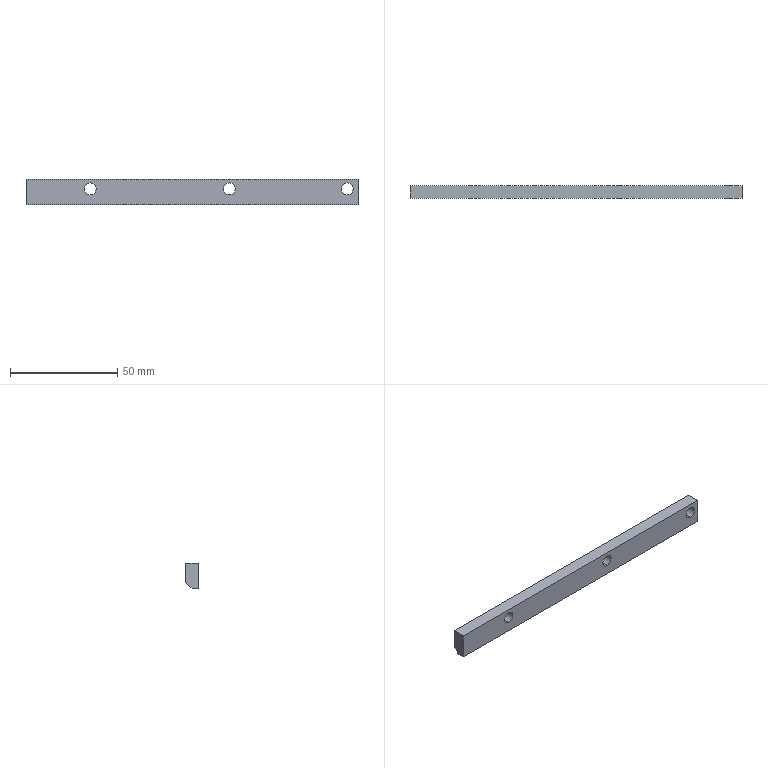Part | STEP file | cover plate 4 | 1 solid | 13 faces | box 155 x 6 x 12 mm | volume 10035 mm3 | plane 7 | cylinder 6 | commonest cylinder face diameters 5.5 x6
STEP:
#1=CARTESIAN_POINT('',(0.,0.,0.));
#2=DIRECTION('',(0.,0.,1.));
#3=DIRECTION('',(1.,0.,0.));
#4=AXIS2_PLACEMENT_3D('',#1,#2,#3);
#5=CARTESIAN_POINT('',(-34.258,0.,9.25));
#6=VERTEX_POINT('',#5);
#7=CARTESIAN_POINT('',(-34.258,6.,9.25));
#8=VERTEX_POINT('',#7);
#9=CARTESIAN_POINT('',(-34.258,6.,9.25));
#10=DIRECTION('',(0.,1.,0.));
#11=VECTOR('',#10,1.);
#12=LINE('',#9,#11);
#13=CARTESIAN_POINT('',(-34.258,6.,6.5));
#14=DIRECTION('',(0.,1.,0.));
#15=DIRECTION('',(0.,0.,1.));
#16=AXIS2_PLACEMENT_3D('',#13,#14,#15);
#17=CYLINDRICAL_SURFACE('',#16,2.75);
#18=CARTESIAN_POINT('',(6.283,0.));
#19=DIRECTION('',(0.,1.));
#20=VECTOR('',#19,1.);
#21=LINE('',#18,#20);
#22=(GEOMETRIC_REPRESENTATION_CONTEXT(2)PARAMETRIC_REPRESENTATION_CONTEXT()REPRESENTATION_CONTEXT('',''));
#23=DEFINITIONAL_REPRESENTATION('',(#21),#22);
#24=PCURVE('',#17,#23);
#25=CARTESIAN_POINT('',(-34.258,6.,6.5));
#26=DIRECTION('',(0.,1.,0.));
#27=DIRECTION('',(0.,0.,1.));
#28=AXIS2_PLACEMENT_3D('',#25,#26,#27);
#29=CYLINDRICAL_SURFACE('',#28,2.75);
#30=CARTESIAN_POINT('',(0.,0.));
#31=DIRECTION('',(0.,1.));
#32=VECTOR('',#31,1.);
#33=LINE('',#30,#32);
#34=(GEOMETRIC_REPRESENTATION_CONTEXT(2)PARAMETRIC_REPRESENTATION_CONTEXT()REPRESENTATION_CONTEXT('',''));
#35=DEFINITIONAL_REPRESENTATION('',(#33),#34);
#36=PCURVE('',#29,#35);
#37=SURFACE_CURVE('',#12,(#24,#36),.PCURVE_S1.);
#38=EDGE_CURVE('',#6,#8,#37,.T.);
#39=ORIENTED_EDGE('',*,*,#38,.T.);
#40=CARTESIAN_POINT('',(-34.258,6.,3.75));
#41=VERTEX_POINT('',#40);
#42=CARTESIAN_POINT('',(-34.258,6.,6.5));
#43=DIRECTION('',(0.,1.,0.));
#44=DIRECTION('',(0.,0.,1.));
#45=AXIS2_PLACEMENT_3D('',#42,#43,#44);
#46=CIRCLE('',#45,2.75);
#47=CARTESIAN_POINT('',(0.,0.));
#48=DIRECTION('',(1.,0.));
#49=VECTOR('',#48,1.);
#50=LINE('',#47,#49);
#51=(GEOMETRIC_REPRESENTATION_CONTEXT(2)PARAMETRIC_REPRESENTATION_CONTEXT()REPRESENTATION_CONTEXT('',''));
#52=DEFINITIONAL_REPRESENTATION('',(#50),#51);
#53=PCURVE('',#17,#52);
#54=CARTESIAN_POINT('',(15.742,6.,11.));
#55=DIRECTION('',(0.,1.,0.));
#56=DIRECTION('',(0.,0.,1.));
#57=AXIS2_PLACEMENT_3D('',#54,#55,#56);
#58=PLANE('',#57);
#59=CARTESIAN_POINT('',(-4.5,-50.));
#60=DIRECTION('',(1.,0.));
#61=AXIS2_PLACEMENT_2D('',#59,#60);
#62=CIRCLE('',#61,2.75);
#63=(GEOMETRIC_REPRESENTATION_CONTEXT(2)PARAMETRIC_REPRESENTATION_CONTEXT()REPRESENTATION_CONTEXT('',''));
#64=DEFINITIONAL_REPRESENTATION('',(#62),#63);
#65=PCURVE('',#58,#64);
#66=SURFACE_CURVE('',#46,(#53,#65),.PCURVE_S1.);
#67=EDGE_CURVE('',#41,#8,#66,.T.);
#68=ORIENTED_EDGE('',*,*,#67,.F.);
#69=CARTESIAN_POINT('',(-34.258,0.,3.75));
#70=VERTEX_POINT('',#69);
#71=CARTESIAN_POINT('',(-34.258,6.,3.75));
#72=DIRECTION('',(0.,1.,0.));
#73=VECTOR('',#72,1.);
#74=LINE('',#71,#73);
#75=CARTESIAN_POINT('',(3.142,0.));
#76=DIRECTION('',(0.,1.));
#77=VECTOR('',#76,1.);
#78=LINE('',#75,#77);
#79=(GEOMETRIC_REPRESENTATION_CONTEXT(2)PARAMETRIC_REPRESENTATION_CONTEXT()REPRESENTATION_CONTEXT('',''));
#80=DEFINITIONAL_REPRESENTATION('',(#78),#79);
#81=PCURVE('',#17,#80);
#82=CARTESIAN_POINT('',(3.142,0.));
#83=DIRECTION('',(0.,1.));
#84=VECTOR('',#83,1.);
#85=LINE('',#82,#84);
#86=(GEOMETRIC_REPRESENTATION_CONTEXT(2)PARAMETRIC_REPRESENTATION_CONTEXT()REPRESENTATION_CONTEXT('',''));
#87=DEFINITIONAL_REPRESENTATION('',(#85),#86);
#88=PCURVE('',#29,#87);
#89=SURFACE_CURVE('',#74,(#81,#88),.PCURVE_S1.);
#90=EDGE_CURVE('',#70,#41,#89,.T.);
#91=ORIENTED_EDGE('',*,*,#90,.F.);
#92=CARTESIAN_POINT('',(-34.258,0.,6.5));
#93=DIRECTION('',(0.,1.,0.));
#94=DIRECTION('',(0.,0.,1.));
#95=AXIS2_PLACEMENT_3D('',#92,#93,#94);
#96=CIRCLE('',#95,2.75);
#97=CARTESIAN_POINT('',(0.,-6.));
#98=DIRECTION('',(1.,0.));
#99=VECTOR('',#98,1.);
#100=LINE('',#97,#99);
#101=(GEOMETRIC_REPRESENTATION_CONTEXT(2)PARAMETRIC_REPRESENTATION_CONTEXT()REPRESENTATION_CONTEXT('',''));
#102=DEFINITIONAL_REPRESENTATION('',(#100),#101);
#103=PCURVE('',#17,#102);
#104=CARTESIAN_POINT('',(15.742,0.,11.));
#105=DIRECTION('',(0.,1.,0.));
#106=DIRECTION('',(0.,0.,1.));
#107=AXIS2_PLACEMENT_3D('',#104,#105,#106);
#108=PLANE('',#107);
#109=CARTESIAN_POINT('',(-4.5,-50.));
#110=DIRECTION('',(1.,0.));
#111=AXIS2_PLACEMENT_2D('',#109,#110);
#112=CIRCLE('',#111,2.75);
#113=(GEOMETRIC_REPRESENTATION_CONTEXT(2)PARAMETRIC_REPRESENTATION_CONTEXT()REPRESENTATION_CONTEXT('',''));
#114=DEFINITIONAL_REPRESENTATION('',(#112),#113);
#115=PCURVE('',#108,#114);
#116=SURFACE_CURVE('',#96,(#103,#115),.PCURVE_S1.);
#117=EDGE_CURVE('',#70,#6,#116,.T.);
#118=ORIENTED_EDGE('',*,*,#117,.T.);
#119=EDGE_LOOP('',(#39,#68,#91,#118));
#120=FACE_BOUND('',#119,.F.);
#121=ADVANCED_FACE('',(#120),#17,.F.);
#122=CARTESIAN_POINT('',(85.742,0.,9.25));
#123=VERTEX_POINT('',#122);
#124=CARTESIAN_POINT('',(85.742,6.,9.25));
#125=VERTEX_POINT('',#124);
#126=CARTESIAN_POINT('',(85.742,6.,9.25));
#127=DIRECTION('',(0.,1.,0.));
#128=VECTOR('',#127,1.);
#129=LINE('',#126,#128);
#130=CARTESIAN_POINT('',(85.742,6.,6.5));
#131=DIRECTION('',(0.,1.,0.));
#132=DIRECTION('',(0.,0.,1.));
#133=AXIS2_PLACEMENT_3D('',#130,#131,#132);
#134=CYLINDRICAL_SURFACE('',#133,2.75);
#135=CARTESIAN_POINT('',(6.283,0.));
#136=DIRECTION('',(0.,1.));
#137=VECTOR('',#136,1.);
#138=LINE('',#135,#137);
#139=(GEOMETRIC_REPRESENTATION_CONTEXT(2)PARAMETRIC_REPRESENTATION_CONTEXT()REPRESENTATION_CONTEXT('',''));
#140=DEFINITIONAL_REPRESENTATION('',(#138),#139);
#141=PCURVE('',#134,#140);
#142=CARTESIAN_POINT('',(85.742,6.,6.5));
#143=DIRECTION('',(0.,1.,0.));
#144=DIRECTION('',(0.,0.,1.));
#145=AXIS2_PLACEMENT_3D('',#142,#143,#144);
#146=CYLINDRICAL_SURFACE('',#145,2.75);
#147=CARTESIAN_POINT('',(0.,0.));
#148=DIRECTION('',(0.,1.));
#149=VECTOR('',#148,1.);
#150=LINE('',#147,#149);
#151=(GEOMETRIC_REPRESENTATION_CONTEXT(2)PARAMETRIC_REPRESENTATION_CONTEXT()REPRESENTATION_CONTEXT('',''));
#152=DEFINITIONAL_REPRESENTATION('',(#150),#151);
#153=PCURVE('',#146,#152);
#154=SURFACE_CURVE('',#129,(#141,#153),.PCURVE_S1.);
#155=EDGE_CURVE('',#123,#125,#154,.T.);
#156=ORIENTED_EDGE('',*,*,#155,.T.);
#157=CARTESIAN_POINT('',(85.742,6.,3.75));
#158=VERTEX_POINT('',#157);
#159=CARTESIAN_POINT('',(85.742,6.,6.5));
#160=DIRECTION('',(0.,1.,0.));
#161=DIRECTION('',(0.,0.,1.));
#162=AXIS2_PLACEMENT_3D('',#159,#160,#161);
#163=CIRCLE('',#162,2.75);
#164=CARTESIAN_POINT('',(0.,0.));
#165=DIRECTION('',(1.,0.));
#166=VECTOR('',#165,1.);
#167=LINE('',#164,#166);
#168=(GEOMETRIC_REPRESENTATION_CONTEXT(2)PARAMETRIC_REPRESENTATION_CONTEXT()REPRESENTATION_CONTEXT('',''));
#169=DEFINITIONAL_REPRESENTATION('',(#167),#168);
#170=PCURVE('',#134,#169);
#171=CARTESIAN_POINT('',(-4.5,70.));
#172=DIRECTION('',(1.,0.));
#173=AXIS2_PLACEMENT_2D('',#171,#172);
#174=CIRCLE('',#173,2.75);
#175=(GEOMETRIC_REPRESENTATION_CONTEXT(2)PARAMETRIC_REPRESENTATION_CONTEXT()REPRESENTATION_CONTEXT('',''));
#176=DEFINITIONAL_REPRESENTATION('',(#174),#175);
#177=PCURVE('',#58,#176);
#178=SURFACE_CURVE('',#163,(#170,#177),.PCURVE_S1.);
#179=EDGE_CURVE('',#158,#125,#178,.T.);
#180=ORIENTED_EDGE('',*,*,#179,.F.);
#181=CARTESIAN_POINT('',(85.742,0.,3.75));
#182=VERTEX_POINT('',#181);
#183=CARTESIAN_POINT('',(85.742,6.,3.75));
#184=DIRECTION('',(0.,1.,0.));
#185=VECTOR('',#184,1.);
#186=LINE('',#183,#185);
#187=CARTESIAN_POINT('',(3.142,0.));
#188=DIRECTION('',(0.,1.));
#189=VECTOR('',#188,1.);
#190=LINE('',#187,#189);
#191=(GEOMETRIC_REPRESENTATION_CONTEXT(2)PARAMETRIC_REPRESENTATION_CONTEXT()REPRESENTATION_CONTEXT('',''));
#192=DEFINITIONAL_REPRESENTATION('',(#190),#191);
#193=PCURVE('',#134,#192);
#194=CARTESIAN_POINT('',(3.142,0.));
#195=DIRECTION('',(0.,1.));
#196=VECTOR('',#195,1.);
#197=LINE('',#194,#196);
#198=(GEOMETRIC_REPRESENTATION_CONTEXT(2)PARAMETRIC_REPRESENTATION_CONTEXT()REPRESENTATION_CONTEXT('',''));
#199=DEFINITIONAL_REPRESENTATION('',(#197),#198);
#200=PCURVE('',#146,#199);
#201=SURFACE_CURVE('',#186,(#193,#200),.PCURVE_S1.);
#202=EDGE_CURVE('',#182,#158,#201,.T.);
#203=ORIENTED_EDGE('',*,*,#202,.F.);
#204=CARTESIAN_POINT('',(85.742,0.,6.5));
#205=DIRECTION('',(0.,1.,0.));
#206=DIRECTION('',(0.,0.,1.));
#207=AXIS2_PLACEMENT_3D('',#204,#205,#206);
#208=CIRCLE('',#207,2.75);
#209=CARTESIAN_POINT('',(0.,-6.));
#210=DIRECTION('',(1.,0.));
#211=VECTOR('',#210,1.);
#212=LINE('',#209,#211);
#213=(GEOMETRIC_REPRESENTATION_CONTEXT(2)PARAMETRIC_REPRESENTATION_CONTEXT()REPRESENTATION_CONTEXT('',''));
#214=DEFINITIONAL_REPRESENTATION('',(#212),#213);
#215=PCURVE('',#134,#214);
#216=CARTESIAN_POINT('',(-4.5,70.));
#217=DIRECTION('',(1.,0.));
#218=AXIS2_PLACEMENT_2D('',#216,#217);
#219=CIRCLE('',#218,2.75);
#220=(GEOMETRIC_REPRESENTATION_CONTEXT(2)PARAMETRIC_REPRESENTATION_CONTEXT()REPRESENTATION_CONTEXT('',''));
#221=DEFINITIONAL_REPRESENTATION('',(#219),#220);
#222=PCURVE('',#108,#221);
#223=SURFACE_CURVE('',#208,(#215,#222),.PCURVE_S1.);
#224=EDGE_CURVE('',#182,#123,#223,.T.);
#225=ORIENTED_EDGE('',*,*,#224,.T.);
#226=EDGE_LOOP('',(#156,#180,#203,#225));
#227=FACE_BOUND('',#226,.F.);
#228=ADVANCED_FACE('',(#227),#134,.F.);
#229=CARTESIAN_POINT('',(30.742,0.,9.25));
#230=VERTEX_POINT('',#229);
#231=CARTESIAN_POINT('',(30.742,6.,9.25));
#232=VERTEX_POINT('',#231);
#233=CARTESIAN_POINT('',(30.742,6.,9.25));
#234=DIRECTION('',(0.,1.,0.));
#235=VECTOR('',#234,1.);
#236=LINE('',#233,#235);
#237=CARTESIAN_POINT('',(30.742,6.,6.5));
#238=DIRECTION('',(0.,1.,0.));
#239=DIRECTION('',(0.,0.,1.));
#240=AXIS2_PLACEMENT_3D('',#237,#238,#239);
#241=CYLINDRICAL_SURFACE('',#240,2.75);
#242=CARTESIAN_POINT('',(6.283,0.));
#243=DIRECTION('',(0.,1.));
#244=VECTOR('',#243,1.);
#245=LINE('',#242,#244);
#246=(GEOMETRIC_REPRESENTATION_CONTEXT(2)PARAMETRIC_REPRESENTATION_CONTEXT()REPRESENTATION_CONTEXT('',''));
#247=DEFINITIONAL_REPRESENTATION('',(#245),#246);
#248=PCURVE('',#241,#247);
#249=CARTESIAN_POINT('',(30.742,6.,6.5));
#250=DIRECTION('',(0.,1.,0.));
#251=DIRECTION('',(0.,0.,1.));
#252=AXIS2_PLACEMENT_3D('',#249,#250,#251);
#253=CYLINDRICAL_SURFACE('',#252,2.75);
#254=CARTESIAN_POINT('',(0.,0.));
#255=DIRECTION('',(0.,1.));
#256=VECTOR('',#255,1.);
#257=LINE('',#254,#256);
#258=(GEOMETRIC_REPRESENTATION_CONTEXT(2)PARAMETRIC_REPRESENTATION_CONTEXT()REPRESENTATION_CONTEXT('',''));
#259=DEFINITIONAL_REPRESENTATION('',(#257),#258);
#260=PCURVE('',#253,#259);
#261=SURFACE_CURVE('',#236,(#248,#260),.PCURVE_S1.);
#262=EDGE_CURVE('',#230,#232,#261,.T.);
#263=ORIENTED_EDGE('',*,*,#262,.T.);
#264=CARTESIAN_POINT('',(30.742,6.,3.75));
#265=VERTEX_POINT('',#264);
#266=CARTESIAN_POINT('',(30.742,6.,6.5));
#267=DIRECTION('',(0.,1.,0.));
#268=DIRECTION('',(0.,0.,1.));
#269=AXIS2_PLACEMENT_3D('',#266,#267,#268);
#270=CIRCLE('',#269,2.75);
#271=CARTESIAN_POINT('',(0.,0.));
#272=DIRECTION('',(1.,0.));
#273=VECTOR('',#272,1.);
#274=LINE('',#271,#273);
#275=(GEOMETRIC_REPRESENTATION_CONTEXT(2)PARAMETRIC_REPRESENTATION_CONTEXT()REPRESENTATION_CONTEXT('',''));
#276=DEFINITIONAL_REPRESENTATION('',(#274),#275);
#277=PCURVE('',#241,#276);
#278=CARTESIAN_POINT('',(-4.5,15.));
#279=DIRECTION('',(1.,0.));
#280=AXIS2_PLACEMENT_2D('',#278,#279);
#281=CIRCLE('',#280,2.75);
#282=(GEOMETRIC_REPRESENTATION_CONTEXT(2)PARAMETRIC_REPRESENTATION_CONTEXT()REPRESENTATION_CONTEXT('',''));
#283=DEFINITIONAL_REPRESENTATION('',(#281),#282);
#284=PCURVE('',#58,#283);
#285=SURFACE_CURVE('',#270,(#277,#284),.PCURVE_S1.);
#286=EDGE_CURVE('',#265,#232,#285,.T.);
#287=ORIENTED_EDGE('',*,*,#286,.F.);
#288=CARTESIAN_POINT('',(30.742,0.,3.75));
#289=VERTEX_POINT('',#288);
#290=CARTESIAN_POINT('',(30.742,6.,3.75));
#291=DIRECTION('',(0.,1.,0.));
#292=VECTOR('',#291,1.);
#293=LINE('',#290,#292);
#294=CARTESIAN_POINT('',(3.142,0.));
#295=DIRECTION('',(0.,1.));
#296=VECTOR('',#295,1.);
#297=LINE('',#294,#296);
#298=(GEOMETRIC_REPRESENTATION_CONTEXT(2)PARAMETRIC_REPRESENTATION_CONTEXT()REPRESENTATION_CONTEXT('',''));
#299=DEFINITIONAL_REPRESENTATION('',(#297),#298);
#300=PCURVE('',#241,#299);
#301=CARTESIAN_POINT('',(3.142,0.));
#302=DIRECTION('',(0.,1.));
#303=VECTOR('',#302,1.);
#304=LINE('',#301,#303);
#305=(GEOMETRIC_REPRESENTATION_CONTEXT(2)PARAMETRIC_REPRESENTATION_CONTEXT()REPRESENTATION_CONTEXT('',''));
#306=DEFINITIONAL_REPRESENTATION('',(#304),#305);
#307=PCURVE('',#253,#306);
#308=SURFACE_CURVE('',#293,(#300,#307),.PCURVE_S1.);
#309=EDGE_CURVE('',#289,#265,#308,.T.);
#310=ORIENTED_EDGE('',*,*,#309,.F.);
#311=CARTESIAN_POINT('',(30.742,0.,6.5));
#312=DIRECTION('',(0.,1.,0.));
#313=DIRECTION('',(0.,0.,1.));
#314=AXIS2_PLACEMENT_3D('',#311,#312,#313);
#315=CIRCLE('',#314,2.75);
#316=CARTESIAN_POINT('',(0.,-6.));
#317=DIRECTION('',(1.,0.));
#318=VECTOR('',#317,1.);
#319=LINE('',#316,#318);
#320=(GEOMETRIC_REPRESENTATION_CONTEXT(2)PARAMETRIC_REPRESENTATION_CONTEXT()REPRESENTATION_CONTEXT('',''));
#321=DEFINITIONAL_REPRESENTATION('',(#319),#320);
#322=PCURVE('',#241,#321);
#323=CARTESIAN_POINT('',(-4.5,15.));
#324=DIRECTION('',(1.,0.));
#325=AXIS2_PLACEMENT_2D('',#323,#324);
#326=CIRCLE('',#325,2.75);
#327=(GEOMETRIC_REPRESENTATION_CONTEXT(2)PARAMETRIC_REPRESENTATION_CONTEXT()REPRESENTATION_CONTEXT('',''));
#328=DEFINITIONAL_REPRESENTATION('',(#326),#327);
#329=PCURVE('',#108,#328);
#330=SURFACE_CURVE('',#315,(#322,#329),.PCURVE_S1.);
#331=EDGE_CURVE('',#289,#230,#330,.T.);
#332=ORIENTED_EDGE('',*,*,#331,.T.);
#333=EDGE_LOOP('',(#263,#287,#310,#332));
#334=FACE_BOUND('',#333,.F.);
#335=ADVANCED_FACE('',(#334),#241,.F.);
#336=CARTESIAN_POINT('',(-64.258,0.,11.));
#337=VERTEX_POINT('',#336);
#338=CARTESIAN_POINT('',(90.742,0.,11.));
#339=VERTEX_POINT('',#338);
#340=CARTESIAN_POINT('',(15.742,0.,11.));
#341=DIRECTION('',(1.,0.,0.));
#342=VECTOR('',#341,1.);
#343=LINE('',#340,#342);
#344=CARTESIAN_POINT('',(15.742,6.,11.));
#345=DIRECTION('',(0.,0.,-1.));
#346=DIRECTION('',(-1.,0.,0.));
#347=AXIS2_PLACEMENT_3D('',#344,#345,#346);
#348=PLANE('',#347);
#349=CARTESIAN_POINT('',(0.,-6.));
#350=DIRECTION('',(-1.,0.));
#351=VECTOR('',#350,1.);
#352=LINE('',#349,#351);
#353=(GEOMETRIC_REPRESENTATION_CONTEXT(2)PARAMETRIC_REPRESENTATION_CONTEXT()REPRESENTATION_CONTEXT('',''));
#354=DEFINITIONAL_REPRESENTATION('',(#352),#353);
#355=PCURVE('',#348,#354);
#356=CARTESIAN_POINT('',(0.,0.));
#357=DIRECTION('',(0.,1.));
#358=VECTOR('',#357,1.);
#359=LINE('',#356,#358);
#360=(GEOMETRIC_REPRESENTATION_CONTEXT(2)PARAMETRIC_REPRESENTATION_CONTEXT()REPRESENTATION_CONTEXT('',''));
#361=DEFINITIONAL_REPRESENTATION('',(#359),#360);
#362=PCURVE('',#108,#361);
#363=SURFACE_CURVE('',#343,(#355,#362),.PCURVE_S1.);
#364=EDGE_CURVE('',#337,#339,#363,.T.);
#365=ORIENTED_EDGE('',*,*,#364,.T.);
#366=CARTESIAN_POINT('',(90.742,6.,11.));
#367=VERTEX_POINT('',#366);
#368=CARTESIAN_POINT('',(90.742,6.,11.));
#369=DIRECTION('',(0.,-1.,0.));
#370=VECTOR('',#369,1.);
#371=LINE('',#368,#370);
#372=CARTESIAN_POINT('',(-75.,0.));
#373=DIRECTION('',(0.,-1.));
#374=VECTOR('',#373,1.);
#375=LINE('',#372,#374);
#376=(GEOMETRIC_REPRESENTATION_CONTEXT(2)PARAMETRIC_REPRESENTATION_CONTEXT()REPRESENTATION_CONTEXT('',''));
#377=DEFINITIONAL_REPRESENTATION('',(#375),#376);
#378=PCURVE('',#348,#377);
#379=CARTESIAN_POINT('',(90.742,0.,-1.));
#380=DIRECTION('',(1.,0.,0.));
#381=DIRECTION('',(0.,0.,-1.));
#382=AXIS2_PLACEMENT_3D('',#379,#380,#381);
#383=PLANE('',#382);
#384=CARTESIAN_POINT('',(-12.,6.));
#385=DIRECTION('',(0.,-1.));
#386=VECTOR('',#385,1.);
#387=LINE('',#384,#386);
#388=(GEOMETRIC_REPRESENTATION_CONTEXT(2)PARAMETRIC_REPRESENTATION_CONTEXT()REPRESENTATION_CONTEXT('',''));
#389=DEFINITIONAL_REPRESENTATION('',(#387),#388);
#390=PCURVE('',#383,#389);
#391=SURFACE_CURVE('',#371,(#378,#390),.PCURVE_S1.);
#392=EDGE_CURVE('',#367,#339,#391,.T.);
#393=ORIENTED_EDGE('',*,*,#392,.F.);
#394=CARTESIAN_POINT('',(-64.258,6.,11.));
#395=VERTEX_POINT('',#394);
#396=CARTESIAN_POINT('',(15.742,6.,11.));
#397=DIRECTION('',(1.,0.,0.));
#398=VECTOR('',#397,1.);
#399=LINE('',#396,#398);
#400=CARTESIAN_POINT('',(0.,0.));
#401=DIRECTION('',(-1.,0.));
#402=VECTOR('',#401,1.);
#403=LINE('',#400,#402);
#404=(GEOMETRIC_REPRESENTATION_CONTEXT(2)PARAMETRIC_REPRESENTATION_CONTEXT()REPRESENTATION_CONTEXT('',''));
#405=DEFINITIONAL_REPRESENTATION('',(#403),#404);
#406=PCURVE('',#348,#405);
#407=CARTESIAN_POINT('',(0.,0.));
#408=DIRECTION('',(0.,1.));
#409=VECTOR('',#408,1.);
#410=LINE('',#407,#409);
#411=(GEOMETRIC_REPRESENTATION_CONTEXT(2)PARAMETRIC_REPRESENTATION_CONTEXT()REPRESENTATION_CONTEXT('',''));
#412=DEFINITIONAL_REPRESENTATION('',(#410),#411);
#413=PCURVE('',#58,#412);
#414=SURFACE_CURVE('',#399,(#406,#413),.PCURVE_S1.);
#415=EDGE_CURVE('',#395,#367,#414,.T.);
#416=ORIENTED_EDGE('',*,*,#415,.F.);
#417=CARTESIAN_POINT('',(-64.258,0.,11.));
#418=DIRECTION('',(0.,1.,0.));
#419=VECTOR('',#418,1.);
#420=LINE('',#417,#419);
#421=CARTESIAN_POINT('',(80.,-6.));
#422=DIRECTION('',(0.,1.));
#423=VECTOR('',#422,1.);
#424=LINE('',#421,#423);
#425=(GEOMETRIC_REPRESENTATION_CONTEXT(2)PARAMETRIC_REPRESENTATION_CONTEXT()REPRESENTATION_CONTEXT('',''));
#426=DEFINITIONAL_REPRESENTATION('',(#424),#425);
#427=PCURVE('',#348,#426);
#428=CARTESIAN_POINT('',(-64.258,6.,11.));
#429=DIRECTION('',(-1.,0.,0.));
#430=DIRECTION('',(0.,0.,1.));
#431=AXIS2_PLACEMENT_3D('',#428,#429,#430);
#432=PLANE('',#431);
#433=CARTESIAN_POINT('',(0.,-6.));
#434=DIRECTION('',(0.,1.));
#435=VECTOR('',#434,1.);
#436=LINE('',#433,#435);
#437=(GEOMETRIC_REPRESENTATION_CONTEXT(2)PARAMETRIC_REPRESENTATION_CONTEXT()REPRESENTATION_CONTEXT('',''));
#438=DEFINITIONAL_REPRESENTATION('',(#436),#437);
#439=PCURVE('',#432,#438);
#440=SURFACE_CURVE('',#420,(#427,#439),.PCURVE_S1.);
#441=EDGE_CURVE('',#337,#395,#440,.T.);
#442=ORIENTED_EDGE('',*,*,#441,.F.);
#443=EDGE_LOOP('',(#365,#393,#416,#442));
#444=FACE_BOUND('',#443,.T.);
#445=ADVANCED_FACE('',(#444),#348,.F.);
#446=CARTESIAN_POINT('',(90.742,0.,-1.));
#447=VERTEX_POINT('',#446);
#448=CARTESIAN_POINT('',(-64.258,0.,-1.));
#449=VERTEX_POINT('',#448);
#450=CARTESIAN_POINT('',(15.742,0.,-1.));
#451=DIRECTION('',(-1.,0.,0.));
#452=VECTOR('',#451,1.);
#453=LINE('',#450,#452);
#454=CARTESIAN_POINT('',(15.742,6.,-1.));
#455=DIRECTION('',(0.,0.,1.));
#456=DIRECTION('',(1.,0.,0.));
#457=AXIS2_PLACEMENT_3D('',#454,#455,#456);
#458=PLANE('',#457);
#459=CARTESIAN_POINT('',(0.,-6.));
#460=DIRECTION('',(-1.,0.));
#461=VECTOR('',#460,1.);
#462=LINE('',#459,#461);
#463=(GEOMETRIC_REPRESENTATION_CONTEXT(2)PARAMETRIC_REPRESENTATION_CONTEXT()REPRESENTATION_CONTEXT('',''));
#464=DEFINITIONAL_REPRESENTATION('',(#462),#463);
#465=PCURVE('',#458,#464);
#466=CARTESIAN_POINT('',(-12.,0.));
#467=DIRECTION('',(0.,-1.));
#468=VECTOR('',#467,1.);
#469=LINE('',#466,#468);
#470=(GEOMETRIC_REPRESENTATION_CONTEXT(2)PARAMETRIC_REPRESENTATION_CONTEXT()REPRESENTATION_CONTEXT('',''));
#471=DEFINITIONAL_REPRESENTATION('',(#469),#470);
#472=PCURVE('',#108,#471);
#473=SURFACE_CURVE('',#453,(#465,#472),.PCURVE_S1.);
#474=EDGE_CURVE('',#447,#449,#473,.T.);
#475=ORIENTED_EDGE('',*,*,#474,.T.);
#476=CARTESIAN_POINT('',(-64.258,3.,-1.));
#477=VERTEX_POINT('',#476);
#478=CARTESIAN_POINT('',(-64.258,3.,-1.));
#479=DIRECTION('',(0.,-1.,0.));
#480=VECTOR('',#479,1.);
#481=LINE('',#478,#480);
#482=CARTESIAN_POINT('',(-80.,-3.));
#483=DIRECTION('',(0.,-1.));
#484=VECTOR('',#483,1.);
#485=LINE('',#482,#484);
#486=(GEOMETRIC_REPRESENTATION_CONTEXT(2)PARAMETRIC_REPRESENTATION_CONTEXT()REPRESENTATION_CONTEXT('',''));
#487=DEFINITIONAL_REPRESENTATION('',(#485),#486);
#488=PCURVE('',#458,#487);
#489=CARTESIAN_POINT('',(-12.,-3.));
#490=DIRECTION('',(0.,-1.));
#491=VECTOR('',#490,1.);
#492=LINE('',#489,#491);
#493=(GEOMETRIC_REPRESENTATION_CONTEXT(2)PARAMETRIC_REPRESENTATION_CONTEXT()REPRESENTATION_CONTEXT('',''));
#494=DEFINITIONAL_REPRESENTATION('',(#492),#493);
#495=PCURVE('',#432,#494);
#496=SURFACE_CURVE('',#481,(#488,#495),.PCURVE_S1.);
#497=EDGE_CURVE('',#477,#449,#496,.T.);
#498=ORIENTED_EDGE('',*,*,#497,.F.);
#499=CARTESIAN_POINT('',(90.742,3.,-1.));
#500=VERTEX_POINT('',#499);
#501=CARTESIAN_POINT('',(60.742,3.,-1.));
#502=DIRECTION('',(1.,0.,0.));
#503=VECTOR('',#502,1.);
#504=LINE('',#501,#503);
#505=CARTESIAN_POINT('',(45.,-3.));
#506=DIRECTION('',(1.,0.));
#507=VECTOR('',#506,1.);
#508=LINE('',#505,#507);
#509=(GEOMETRIC_REPRESENTATION_CONTEXT(2)PARAMETRIC_REPRESENTATION_CONTEXT()REPRESENTATION_CONTEXT('',''));
#510=DEFINITIONAL_REPRESENTATION('',(#508),#509);
#511=PCURVE('',#458,#510);
#512=CARTESIAN_POINT('',(15.742,6.,2.));
#513=DIRECTION('',(0.,0.7071,-0.7071));
#514=DIRECTION('',(0.,0.7071,0.7071));
#515=AXIS2_PLACEMENT_3D('',#512,#513,#514);
#516=PLANE('',#515);
#517=CARTESIAN_POINT('',(-4.243,45.));
#518=DIRECTION('',(0.,1.));
#519=VECTOR('',#518,1.);
#520=LINE('',#517,#519);
#521=(GEOMETRIC_REPRESENTATION_CONTEXT(2)PARAMETRIC_REPRESENTATION_CONTEXT()REPRESENTATION_CONTEXT('',''));
#522=DEFINITIONAL_REPRESENTATION('',(#520),#521);
#523=PCURVE('',#516,#522);
#524=SURFACE_CURVE('',#504,(#511,#523),.PCURVE_S1.);
#525=EDGE_CURVE('',#477,#500,#524,.T.);
#526=ORIENTED_EDGE('',*,*,#525,.T.);
#527=CARTESIAN_POINT('',(90.742,0.,-1.));
#528=DIRECTION('',(0.,1.,0.));
#529=VECTOR('',#528,1.);
#530=LINE('',#527,#529);
#531=CARTESIAN_POINT('',(75.,-6.));
#532=DIRECTION('',(0.,1.));
#533=VECTOR('',#532,1.);
#534=LINE('',#531,#533);
#535=(GEOMETRIC_REPRESENTATION_CONTEXT(2)PARAMETRIC_REPRESENTATION_CONTEXT()REPRESENTATION_CONTEXT('',''));
#536=DEFINITIONAL_REPRESENTATION('',(#534),#535);
#537=PCURVE('',#458,#536);
#538=CARTESIAN_POINT('',(0.,0.));
#539=DIRECTION('',(0.,1.));
#540=VECTOR('',#539,1.);
#541=LINE('',#538,#540);
#542=(GEOMETRIC_REPRESENTATION_CONTEXT(2)PARAMETRIC_REPRESENTATION_CONTEXT()REPRESENTATION_CONTEXT('',''));
#543=DEFINITIONAL_REPRESENTATION('',(#541),#542);
#544=PCURVE('',#383,#543);
#545=SURFACE_CURVE('',#530,(#537,#544),.PCURVE_S1.);
#546=EDGE_CURVE('',#447,#500,#545,.T.);
#547=ORIENTED_EDGE('',*,*,#546,.F.);
#548=EDGE_LOOP('',(#475,#498,#526,#547));
#549=FACE_BOUND('',#548,.T.);
#550=ADVANCED_FACE('',(#549),#458,.F.);
#551=CARTESIAN_POINT('',(-34.258,6.,6.5));
#552=DIRECTION('',(0.,1.,0.));
#553=DIRECTION('',(0.,0.,1.));
#554=AXIS2_PLACEMENT_3D('',#551,#552,#553);
#555=CIRCLE('',#554,2.75);
#556=CARTESIAN_POINT('',(-4.5,-50.));
#557=DIRECTION('',(1.,0.));
#558=AXIS2_PLACEMENT_2D('',#556,#557);
#559=CIRCLE('',#558,2.75);
#560=(GEOMETRIC_REPRESENTATION_CONTEXT(2)PARAMETRIC_REPRESENTATION_CONTEXT()REPRESENTATION_CONTEXT('',''));
#561=DEFINITIONAL_REPRESENTATION('',(#559),#560);
#562=PCURVE('',#58,#561);
#563=CARTESIAN_POINT('',(0.,0.));
#564=DIRECTION('',(1.,0.));
#565=VECTOR('',#564,1.);
#566=LINE('',#563,#565);
#567=(GEOMETRIC_REPRESENTATION_CONTEXT(2)PARAMETRIC_REPRESENTATION_CONTEXT()REPRESENTATION_CONTEXT('',''));
#568=DEFINITIONAL_REPRESENTATION('',(#566),#567);
#569=PCURVE('',#29,#568);
#570=SURFACE_CURVE('',#555,(#562,#569),.PCURVE_S1.);
#571=EDGE_CURVE('',#8,#41,#570,.T.);
#572=ORIENTED_EDGE('',*,*,#571,.F.);
#573=ORIENTED_EDGE('',*,*,#67,.F.);
#574=EDGE_LOOP('',(#572,#573));
#575=FACE_BOUND('',#574,.T.);
#576=CARTESIAN_POINT('',(85.742,6.,6.5));
#577=DIRECTION('',(0.,1.,0.));
#578=DIRECTION('',(0.,0.,1.));
#579=AXIS2_PLACEMENT_3D('',#576,#577,#578);
#580=CIRCLE('',#579,2.75);
#581=CARTESIAN_POINT('',(-4.5,70.));
#582=DIRECTION('',(1.,0.));
#583=AXIS2_PLACEMENT_2D('',#581,#582);
#584=CIRCLE('',#583,2.75);
#585=(GEOMETRIC_REPRESENTATION_CONTEXT(2)PARAMETRIC_REPRESENTATION_CONTEXT()REPRESENTATION_CONTEXT('',''));
#586=DEFINITIONAL_REPRESENTATION('',(#584),#585);
#587=PCURVE('',#58,#586);
#588=CARTESIAN_POINT('',(0.,0.));
#589=DIRECTION('',(1.,0.));
#590=VECTOR('',#589,1.);
#591=LINE('',#588,#590);
#592=(GEOMETRIC_REPRESENTATION_CONTEXT(2)PARAMETRIC_REPRESENTATION_CONTEXT()REPRESENTATION_CONTEXT('',''));
#593=DEFINITIONAL_REPRESENTATION('',(#591),#592);
#594=PCURVE('',#146,#593);
#595=SURFACE_CURVE('',#580,(#587,#594),.PCURVE_S1.);
#596=EDGE_CURVE('',#125,#158,#595,.T.);
#597=ORIENTED_EDGE('',*,*,#596,.F.);
#598=ORIENTED_EDGE('',*,*,#179,.F.);
#599=EDGE_LOOP('',(#597,#598));
#600=FACE_BOUND('',#599,.T.);
#601=CARTESIAN_POINT('',(30.742,6.,6.5));
#602=DIRECTION('',(0.,1.,0.));
#603=DIRECTION('',(0.,0.,1.));
#604=AXIS2_PLACEMENT_3D('',#601,#602,#603);
#605=CIRCLE('',#604,2.75);
#606=CARTESIAN_POINT('',(-4.5,15.));
#607=DIRECTION('',(1.,0.));
#608=AXIS2_PLACEMENT_2D('',#606,#607);
#609=CIRCLE('',#608,2.75);
#610=(GEOMETRIC_REPRESENTATION_CONTEXT(2)PARAMETRIC_REPRESENTATION_CONTEXT()REPRESENTATION_CONTEXT('',''));
#611=DEFINITIONAL_REPRESENTATION('',(#609),#610);
#612=PCURVE('',#58,#611);
#613=CARTESIAN_POINT('',(0.,0.));
#614=DIRECTION('',(1.,0.));
#615=VECTOR('',#614,1.);
#616=LINE('',#613,#615);
#617=(GEOMETRIC_REPRESENTATION_CONTEXT(2)PARAMETRIC_REPRESENTATION_CONTEXT()REPRESENTATION_CONTEXT('',''));
#618=DEFINITIONAL_REPRESENTATION('',(#616),#617);
#619=PCURVE('',#253,#618);
#620=SURFACE_CURVE('',#605,(#612,#619),.PCURVE_S1.);
#621=EDGE_CURVE('',#232,#265,#620,.T.);
#622=ORIENTED_EDGE('',*,*,#621,.F.);
#623=ORIENTED_EDGE('',*,*,#286,.F.);
#624=EDGE_LOOP('',(#622,#623));
#625=FACE_BOUND('',#624,.T.);
#626=ORIENTED_EDGE('',*,*,#415,.T.);
#627=CARTESIAN_POINT('',(90.742,6.,2.));
#628=VERTEX_POINT('',#627);
#629=CARTESIAN_POINT('',(90.742,6.,2.));
#630=DIRECTION('',(0.,0.,1.));
#631=VECTOR('',#630,1.);
#632=LINE('',#629,#631);
#633=CARTESIAN_POINT('',(-9.,75.));
#634=DIRECTION('',(1.,0.));
#635=VECTOR('',#634,1.);
#636=LINE('',#633,#635);
#637=(GEOMETRIC_REPRESENTATION_CONTEXT(2)PARAMETRIC_REPRESENTATION_CONTEXT()REPRESENTATION_CONTEXT('',''));
#638=DEFINITIONAL_REPRESENTATION('',(#636),#637);
#639=PCURVE('',#58,#638);
#640=CARTESIAN_POINT('',(-3.,6.));
#641=DIRECTION('',(-1.,0.));
#642=VECTOR('',#641,1.);
#643=LINE('',#640,#642);
#644=(GEOMETRIC_REPRESENTATION_CONTEXT(2)PARAMETRIC_REPRESENTATION_CONTEXT()REPRESENTATION_CONTEXT('',''));
#645=DEFINITIONAL_REPRESENTATION('',(#643),#644);
#646=PCURVE('',#383,#645);
#647=SURFACE_CURVE('',#632,(#639,#646),.PCURVE_S1.);
#648=EDGE_CURVE('',#628,#367,#647,.T.);
#649=ORIENTED_EDGE('',*,*,#648,.F.);
#650=CARTESIAN_POINT('',(-64.258,6.,2.));
#651=VERTEX_POINT('',#650);
#652=CARTESIAN_POINT('',(15.742,6.,2.));
#653=DIRECTION('',(-1.,0.,0.));
#654=VECTOR('',#653,1.);
#655=LINE('',#652,#654);
#656=CARTESIAN_POINT('',(-9.,0.));
#657=DIRECTION('',(0.,-1.));
#658=VECTOR('',#657,1.);
#659=LINE('',#656,#658);
#660=(GEOMETRIC_REPRESENTATION_CONTEXT(2)PARAMETRIC_REPRESENTATION_CONTEXT()REPRESENTATION_CONTEXT('',''));
#661=DEFINITIONAL_REPRESENTATION('',(#659),#660);
#662=PCURVE('',#58,#661);
#663=CARTESIAN_POINT('',(0.,0.));
#664=DIRECTION('',(0.,-1.));
#665=VECTOR('',#664,1.);
#666=LINE('',#663,#665);
#667=(GEOMETRIC_REPRESENTATION_CONTEXT(2)PARAMETRIC_REPRESENTATION_CONTEXT()REPRESENTATION_CONTEXT('',''));
#668=DEFINITIONAL_REPRESENTATION('',(#666),#667);
#669=PCURVE('',#516,#668);
#670=SURFACE_CURVE('',#655,(#662,#669),.PCURVE_S1.);
#671=EDGE_CURVE('',#628,#651,#670,.T.);
#672=ORIENTED_EDGE('',*,*,#671,.T.);
#673=CARTESIAN_POINT('',(-64.258,6.,11.));
#674=DIRECTION('',(0.,0.,-1.));
#675=VECTOR('',#674,1.);
#676=LINE('',#673,#675);
#677=CARTESIAN_POINT('',(0.,-80.));
#678=DIRECTION('',(-1.,0.));
#679=VECTOR('',#678,1.);
#680=LINE('',#677,#679);
#681=(GEOMETRIC_REPRESENTATION_CONTEXT(2)PARAMETRIC_REPRESENTATION_CONTEXT()REPRESENTATION_CONTEXT('',''));
#682=DEFINITIONAL_REPRESENTATION('',(#680),#681);
#683=PCURVE('',#58,#682);
#684=CARTESIAN_POINT('',(0.,0.));
#685=DIRECTION('',(-1.,0.));
#686=VECTOR('',#685,1.);
#687=LINE('',#684,#686);
#688=(GEOMETRIC_REPRESENTATION_CONTEXT(2)PARAMETRIC_REPRESENTATION_CONTEXT()REPRESENTATION_CONTEXT('',''));
#689=DEFINITIONAL_REPRESENTATION('',(#687),#688);
#690=PCURVE('',#432,#689);
#691=SURFACE_CURVE('',#676,(#683,#690),.PCURVE_S1.);
#692=EDGE_CURVE('',#395,#651,#691,.T.);
#693=ORIENTED_EDGE('',*,*,#692,.F.);
#694=EDGE_LOOP('',(#626,#649,#672,#693));
#695=FACE_BOUND('',#694,.T.);
#696=ADVANCED_FACE('',(#575,#600,#625,#695),#58,.T.);
#697=CARTESIAN_POINT('',(-34.258,0.,6.5));
#698=DIRECTION('',(0.,1.,0.));
#699=DIRECTION('',(0.,0.,1.));
#700=AXIS2_PLACEMENT_3D('',#697,#698,#699);
#701=CIRCLE('',#700,2.75);
#702=CARTESIAN_POINT('',(-4.5,-50.));
#703=DIRECTION('',(1.,0.));
#704=AXIS2_PLACEMENT_2D('',#702,#703);
#705=CIRCLE('',#704,2.75);
#706=(GEOMETRIC_REPRESENTATION_CONTEXT(2)PARAMETRIC_REPRESENTATION_CONTEXT()REPRESENTATION_CONTEXT('',''));
#707=DEFINITIONAL_REPRESENTATION('',(#705),#706);
#708=PCURVE('',#108,#707);
#709=CARTESIAN_POINT('',(0.,-6.));
#710=DIRECTION('',(1.,0.));
#711=VECTOR('',#710,1.);
#712=LINE('',#709,#711);
#713=(GEOMETRIC_REPRESENTATION_CONTEXT(2)PARAMETRIC_REPRESENTATION_CONTEXT()REPRESENTATION_CONTEXT('',''));
#714=DEFINITIONAL_REPRESENTATION('',(#712),#713);
#715=PCURVE('',#29,#714);
#716=SURFACE_CURVE('',#701,(#708,#715),.PCURVE_S1.);
#717=EDGE_CURVE('',#6,#70,#716,.T.);
#718=ORIENTED_EDGE('',*,*,#717,.T.);
#719=ORIENTED_EDGE('',*,*,#117,.T.);
#720=EDGE_LOOP('',(#718,#719));
#721=FACE_BOUND('',#720,.T.);
#722=CARTESIAN_POINT('',(85.742,0.,6.5));
#723=DIRECTION('',(0.,1.,0.));
#724=DIRECTION('',(0.,0.,1.));
#725=AXIS2_PLACEMENT_3D('',#722,#723,#724);
#726=CIRCLE('',#725,2.75);
#727=CARTESIAN_POINT('',(-4.5,70.));
#728=DIRECTION('',(1.,0.));
#729=AXIS2_PLACEMENT_2D('',#727,#728);
#730=CIRCLE('',#729,2.75);
#731=(GEOMETRIC_REPRESENTATION_CONTEXT(2)PARAMETRIC_REPRESENTATION_CONTEXT()REPRESENTATION_CONTEXT('',''));
#732=DEFINITIONAL_REPRESENTATION('',(#730),#731);
#733=PCURVE('',#108,#732);
#734=CARTESIAN_POINT('',(0.,-6.));
#735=DIRECTION('',(1.,0.));
#736=VECTOR('',#735,1.);
#737=LINE('',#734,#736);
#738=(GEOMETRIC_REPRESENTATION_CONTEXT(2)PARAMETRIC_REPRESENTATION_CONTEXT()REPRESENTATION_CONTEXT('',''));
#739=DEFINITIONAL_REPRESENTATION('',(#737),#738);
#740=PCURVE('',#146,#739);
#741=SURFACE_CURVE('',#726,(#733,#740),.PCURVE_S1.);
#742=EDGE_CURVE('',#123,#182,#741,.T.);
#743=ORIENTED_EDGE('',*,*,#742,.T.);
#744=ORIENTED_EDGE('',*,*,#224,.T.);
#745=EDGE_LOOP('',(#743,#744));
#746=FACE_BOUND('',#745,.T.);
#747=CARTESIAN_POINT('',(30.742,0.,6.5));
#748=DIRECTION('',(0.,1.,0.));
#749=DIRECTION('',(0.,0.,1.));
#750=AXIS2_PLACEMENT_3D('',#747,#748,#749);
#751=CIRCLE('',#750,2.75);
#752=CARTESIAN_POINT('',(-4.5,15.));
#753=DIRECTION('',(1.,0.));
#754=AXIS2_PLACEMENT_2D('',#752,#753);
#755=CIRCLE('',#754,2.75);
#756=(GEOMETRIC_REPRESENTATION_CONTEXT(2)PARAMETRIC_REPRESENTATION_CONTEXT()REPRESENTATION_CONTEXT('',''));
#757=DEFINITIONAL_REPRESENTATION('',(#755),#756);
#758=PCURVE('',#108,#757);
#759=CARTESIAN_POINT('',(0.,-6.));
#760=DIRECTION('',(1.,0.));
#761=VECTOR('',#760,1.);
#762=LINE('',#759,#761);
#763=(GEOMETRIC_REPRESENTATION_CONTEXT(2)PARAMETRIC_REPRESENTATION_CONTEXT()REPRESENTATION_CONTEXT('',''));
#764=DEFINITIONAL_REPRESENTATION('',(#762),#763);
#765=PCURVE('',#253,#764);
#766=SURFACE_CURVE('',#751,(#758,#765),.PCURVE_S1.);
#767=EDGE_CURVE('',#230,#289,#766,.T.);
#768=ORIENTED_EDGE('',*,*,#767,.T.);
#769=ORIENTED_EDGE('',*,*,#331,.T.);
#770=EDGE_LOOP('',(#768,#769));
#771=FACE_BOUND('',#770,.T.);
#772=ORIENTED_EDGE('',*,*,#364,.F.);
#773=CARTESIAN_POINT('',(-64.258,0.,-1.));
#774=DIRECTION('',(0.,0.,1.));
#775=VECTOR('',#774,1.);
#776=LINE('',#773,#775);
#777=CARTESIAN_POINT('',(-12.,-80.));
#778=DIRECTION('',(1.,0.));
#779=VECTOR('',#778,1.);
#780=LINE('',#777,#779);
#781=(GEOMETRIC_REPRESENTATION_CONTEXT(2)PARAMETRIC_REPRESENTATION_CONTEXT()REPRESENTATION_CONTEXT('',''));
#782=DEFINITIONAL_REPRESENTATION('',(#780),#781);
#783=PCURVE('',#108,#782);
#784=CARTESIAN_POINT('',(-12.,-6.));
#785=DIRECTION('',(1.,0.));
#786=VECTOR('',#785,1.);
#787=LINE('',#784,#786);
#788=(GEOMETRIC_REPRESENTATION_CONTEXT(2)PARAMETRIC_REPRESENTATION_CONTEXT()REPRESENTATION_CONTEXT('',''));
#789=DEFINITIONAL_REPRESENTATION('',(#787),#788);
#790=PCURVE('',#432,#789);
#791=SURFACE_CURVE('',#776,(#783,#790),.PCURVE_S1.);
#792=EDGE_CURVE('',#449,#337,#791,.T.);
#793=ORIENTED_EDGE('',*,*,#792,.F.);
#794=ORIENTED_EDGE('',*,*,#474,.F.);
#795=CARTESIAN_POINT('',(90.742,0.,11.));
#796=DIRECTION('',(0.,0.,-1.));
#797=VECTOR('',#796,1.);
#798=LINE('',#795,#797);
#799=CARTESIAN_POINT('',(0.,75.));
#800=DIRECTION('',(-1.,0.));
#801=VECTOR('',#800,1.);
#802=LINE('',#799,#801);
#803=(GEOMETRIC_REPRESENTATION_CONTEXT(2)PARAMETRIC_REPRESENTATION_CONTEXT()REPRESENTATION_CONTEXT('',''));
#804=DEFINITIONAL_REPRESENTATION('',(#802),#803);
#805=PCURVE('',#108,#804);
#806=CARTESIAN_POINT('',(-12.,0.));
#807=DIRECTION('',(1.,0.));
#808=VECTOR('',#807,1.);
#809=LINE('',#806,#808);
#810=(GEOMETRIC_REPRESENTATION_CONTEXT(2)PARAMETRIC_REPRESENTATION_CONTEXT()REPRESENTATION_CONTEXT('',''));
#811=DEFINITIONAL_REPRESENTATION('',(#809),#810);
#812=PCURVE('',#383,#811);
#813=SURFACE_CURVE('',#798,(#805,#812),.PCURVE_S1.);
#814=EDGE_CURVE('',#339,#447,#813,.T.);
#815=ORIENTED_EDGE('',*,*,#814,.F.);
#816=EDGE_LOOP('',(#772,#793,#794,#815));
#817=FACE_BOUND('',#816,.T.);
#818=ADVANCED_FACE('',(#721,#746,#771,#817),#108,.F.);
#819=ORIENTED_EDGE('',*,*,#671,.F.);
#820=CARTESIAN_POINT('',(90.742,3.,-1.));
#821=DIRECTION('',(0.,0.7071,0.7071));
#822=VECTOR('',#821,1.);
#823=LINE('',#820,#822);
#824=CARTESIAN_POINT('',(-4.243,75.));
#825=DIRECTION('',(1.,0.));
#826=VECTOR('',#825,1.);
#827=LINE('',#824,#826);
#828=(GEOMETRIC_REPRESENTATION_CONTEXT(2)PARAMETRIC_REPRESENTATION_CONTEXT()REPRESENTATION_CONTEXT('',''));
#829=DEFINITIONAL_REPRESENTATION('',(#827),#828);
#830=PCURVE('',#516,#829);
#831=CARTESIAN_POINT('',(0.,3.));
#832=DIRECTION('',(-0.7071,0.7071));
#833=VECTOR('',#832,1.);
#834=LINE('',#831,#833);
#835=(GEOMETRIC_REPRESENTATION_CONTEXT(2)PARAMETRIC_REPRESENTATION_CONTEXT()REPRESENTATION_CONTEXT('',''));
#836=DEFINITIONAL_REPRESENTATION('',(#834),#835);
#837=PCURVE('',#383,#836);
#838=SURFACE_CURVE('',#823,(#830,#837),.PCURVE_S1.);
#839=EDGE_CURVE('',#500,#628,#838,.T.);
#840=ORIENTED_EDGE('',*,*,#839,.F.);
#841=ORIENTED_EDGE('',*,*,#525,.F.);
#842=CARTESIAN_POINT('',(-64.258,6.,2.));
#843=DIRECTION('',(0.,-0.7071,-0.7071));
#844=VECTOR('',#843,1.);
#845=LINE('',#842,#844);
#846=CARTESIAN_POINT('',(0.,-80.));
#847=DIRECTION('',(-1.,0.));
#848=VECTOR('',#847,1.);
#849=LINE('',#846,#848);
#850=(GEOMETRIC_REPRESENTATION_CONTEXT(2)PARAMETRIC_REPRESENTATION_CONTEXT()REPRESENTATION_CONTEXT('',''));
#851=DEFINITIONAL_REPRESENTATION('',(#849),#850);
#852=PCURVE('',#516,#851);
#853=CARTESIAN_POINT('',(-9.,0.));
#854=DIRECTION('',(-0.7071,-0.7071));
#855=VECTOR('',#854,1.);
#856=LINE('',#853,#855);
#857=(GEOMETRIC_REPRESENTATION_CONTEXT(2)PARAMETRIC_REPRESENTATION_CONTEXT()REPRESENTATION_CONTEXT('',''));
#858=DEFINITIONAL_REPRESENTATION('',(#856),#857);
#859=PCURVE('',#432,#858);
#860=SURFACE_CURVE('',#845,(#852,#859),.PCURVE_S1.);
#861=EDGE_CURVE('',#651,#477,#860,.T.);
#862=ORIENTED_EDGE('',*,*,#861,.F.);
#863=EDGE_LOOP('',(#819,#840,#841,#862));
#864=FACE_BOUND('',#863,.T.);
#865=ADVANCED_FACE('',(#864),#516,.T.);
#866=ORIENTED_EDGE('',*,*,#621,.F.);
#867=ORIENTED_EDGE('',*,*,#262,.F.);
#868=ORIENTED_EDGE('',*,*,#767,.T.);
#869=ORIENTED_EDGE('',*,*,#309,.T.);
#870=EDGE_LOOP('',(#866,#867,#868,#869));
#871=FACE_BOUND('',#870,.F.);
#872=ADVANCED_FACE('',(#871),#253,.F.);
#873=ORIENTED_EDGE('',*,*,#441,.T.);
#874=ORIENTED_EDGE('',*,*,#692,.T.);
#875=ORIENTED_EDGE('',*,*,#861,.T.);
#876=ORIENTED_EDGE('',*,*,#497,.T.);
#877=ORIENTED_EDGE('',*,*,#792,.T.);
#878=EDGE_LOOP('',(#873,#874,#875,#876,#877));
#879=FACE_BOUND('',#878,.T.);
#880=ADVANCED_FACE('',(#879),#432,.T.);
#881=ORIENTED_EDGE('',*,*,#814,.T.);
#882=ORIENTED_EDGE('',*,*,#546,.T.);
#883=ORIENTED_EDGE('',*,*,#839,.T.);
#884=ORIENTED_EDGE('',*,*,#648,.T.);
#885=ORIENTED_EDGE('',*,*,#392,.T.);
#886=EDGE_LOOP('',(#881,#882,#883,#884,#885));
#887=FACE_BOUND('',#886,.T.);
#888=ADVANCED_FACE('',(#887),#383,.T.);
#889=ORIENTED_EDGE('',*,*,#596,.F.);
#890=ORIENTED_EDGE('',*,*,#155,.F.);
#891=ORIENTED_EDGE('',*,*,#742,.T.);
#892=ORIENTED_EDGE('',*,*,#202,.T.);
#893=EDGE_LOOP('',(#889,#890,#891,#892));
#894=FACE_BOUND('',#893,.F.);
#895=ADVANCED_FACE('',(#894),#146,.F.);
#896=ORIENTED_EDGE('',*,*,#571,.F.);
#897=ORIENTED_EDGE('',*,*,#38,.F.);
#898=ORIENTED_EDGE('',*,*,#717,.T.);
#899=ORIENTED_EDGE('',*,*,#90,.T.);
#900=EDGE_LOOP('',(#896,#897,#898,#899));
#901=FACE_BOUND('',#900,.F.);
#902=ADVANCED_FACE('',(#901),#29,.F.);
#903=CLOSED_SHELL('',(#121,#228,#335,#445,#550,#696,#818,#865,#872,#880,#888,#895,#902));
#904=MANIFOLD_SOLID_BREP('',#903);
#905=(LENGTH_UNIT()NAMED_UNIT(*)SI_UNIT(.MILLI.,.METRE.));
#906=UNCERTAINTY_MEASURE_WITH_UNIT(LENGTH_MEASURE(0.0000001),#905,'','');
#907=(NAMED_UNIT(*)PLANE_ANGLE_UNIT()SI_UNIT($,.RADIAN.));
#908=(NAMED_UNIT(*)SI_UNIT($,.STERADIAN.)SOLID_ANGLE_UNIT());
#909=(GEOMETRIC_REPRESENTATION_CONTEXT(3)GLOBAL_UNCERTAINTY_ASSIGNED_CONTEXT((#906))GLOBAL_UNIT_ASSIGNED_CONTEXT((#905,#907,#908))REPRESENTATION_CONTEXT('',''));
#910=ADVANCED_BREP_SHAPE_REPRESENTATION('',(#4,#904),#909);